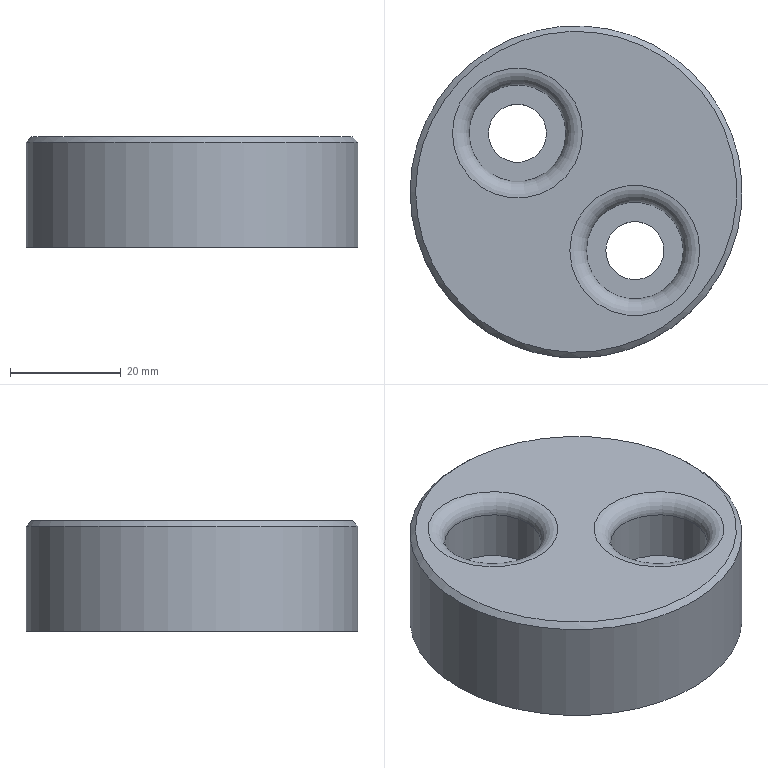Part | NX | features XD1540-60-20 2 | 1 solid | 12 faces | box 60 x 60 x 20 mm | volume 49069 mm3 | cylinder 5 | plane 4 | torus 2 | cone 1 | commonest cylinder face diameters 10.5 x2 17.5 x2 60 x1
STEP:
#1=CARTESIAN_POINT('',(271.,445.,-360.));
#2=VERTEX_POINT('',#1);
#3=CARTESIAN_POINT('',(300.,445.,-360.));
#4=DIRECTION('',(0.,0.,-1.));
#5=DIRECTION('',(-1.,0.,0.));
#6=AXIS2_PLACEMENT_3D('',#3,#4,#5);
#7=CIRCLE('',#6,29.);
#8=EDGE_CURVE('',#2,#2,#7,.T.);
#9=ORIENTED_EDGE('',*,*,#8,.F.);
#10=EDGE_LOOP('',(#9));
#11=FACE_BOUND('',#10,.T.);
#12=CARTESIAN_POINT('',(298.857,434.393,-360.));
#13=VERTEX_POINT('',#12);
#14=CARTESIAN_POINT('',(310.607,434.393,-360.));
#15=DIRECTION('',(0.,0.,1.));
#16=DIRECTION('',(-1.,0.,0.));
#17=AXIS2_PLACEMENT_3D('',#14,#15,#16);
#18=CIRCLE('',#17,11.75);
#19=EDGE_CURVE('',#13,#13,#18,.T.);
#20=ORIENTED_EDGE('',*,*,#19,.F.);
#21=EDGE_LOOP('',(#20));
#22=FACE_BOUND('',#21,.T.);
#23=CARTESIAN_POINT('',(277.643,455.607,-360.));
#24=VERTEX_POINT('',#23);
#25=CARTESIAN_POINT('',(289.393,455.607,-360.));
#26=DIRECTION('',(0.,0.,1.));
#27=DIRECTION('',(-1.,0.,0.));
#28=AXIS2_PLACEMENT_3D('',#25,#26,#27);
#29=CIRCLE('',#28,11.75);
#30=EDGE_CURVE('',#24,#24,#29,.T.);
#31=ORIENTED_EDGE('',*,*,#30,.F.);
#32=EDGE_LOOP('',(#31));
#33=FACE_BOUND('',#32,.T.);
#34=CARTESIAN_POINT('',(300.,445.,-360.));
#35=DIRECTION('',(0.,0.,1.));
#36=DIRECTION('',(1.,0.,0.));
#37=AXIS2_PLACEMENT_3D('',#34,#35,#36);
#38=PLANE('',#37);
#39=ADVANCED_FACE('',(#11,#22,#33),#38,.T.);
#40=CARTESIAN_POINT('',(270.,445.,-380.));
#41=VERTEX_POINT('',#40);
#42=CARTESIAN_POINT('',(300.,445.,-380.));
#43=DIRECTION('',(0.,0.,-1.));
#44=DIRECTION('',(-1.,0.,0.));
#45=AXIS2_PLACEMENT_3D('',#42,#43,#44);
#46=CIRCLE('',#45,30.);
#47=EDGE_CURVE('',#41,#41,#46,.T.);
#48=ORIENTED_EDGE('',*,*,#47,.T.);
#49=EDGE_LOOP('',(#48));
#50=FACE_BOUND('',#49,.T.);
#51=CARTESIAN_POINT('',(315.857,434.393,-380.));
#52=VERTEX_POINT('',#51);
#53=CARTESIAN_POINT('',(310.607,434.393,-380.));
#54=DIRECTION('',(0.,0.,1.));
#55=DIRECTION('',(1.,0.,0.));
#56=AXIS2_PLACEMENT_3D('',#53,#54,#55);
#57=CIRCLE('',#56,5.25);
#58=EDGE_CURVE('',#52,#52,#57,.T.);
#59=ORIENTED_EDGE('',*,*,#58,.T.);
#60=EDGE_LOOP('',(#59));
#61=FACE_BOUND('',#60,.T.);
#62=CARTESIAN_POINT('',(294.643,455.607,-380.));
#63=VERTEX_POINT('',#62);
#64=CARTESIAN_POINT('',(289.393,455.607,-380.));
#65=DIRECTION('',(0.,0.,1.));
#66=DIRECTION('',(1.,0.,0.));
#67=AXIS2_PLACEMENT_3D('',#64,#65,#66);
#68=CIRCLE('',#67,5.25);
#69=EDGE_CURVE('',#63,#63,#68,.T.);
#70=ORIENTED_EDGE('',*,*,#69,.T.);
#71=EDGE_LOOP('',(#70));
#72=FACE_BOUND('',#71,.T.);
#73=CARTESIAN_POINT('',(300.,445.,-380.));
#74=DIRECTION('',(0.,0.,-1.));
#75=DIRECTION('',(-1.,0.,0.));
#76=AXIS2_PLACEMENT_3D('',#73,#74,#75);
#77=PLANE('',#76);
#78=ADVANCED_FACE('',(#50,#61,#72),#77,.T.);
#79=CARTESIAN_POINT('',(325.937,429.925,-361.));
#80=VERTEX_POINT('',#79);
#81=CARTESIAN_POINT('',(300.,445.,-361.));
#82=DIRECTION('',(0.,0.,1.));
#83=DIRECTION('',(-1.,0.,0.));
#84=AXIS2_PLACEMENT_3D('',#81,#82,#83);
#85=CIRCLE('',#84,30.);
#86=EDGE_CURVE('',#80,#80,#85,.T.);
#87=ORIENTED_EDGE('',*,*,#86,.F.);
#88=EDGE_LOOP('',(#87));
#89=FACE_BOUND('',#88,.T.);
#90=ORIENTED_EDGE('',*,*,#47,.F.);
#91=EDGE_LOOP('',(#90));
#92=FACE_BOUND('',#91,.T.);
#93=CARTESIAN_POINT('',(300.,445.,-380.));
#94=DIRECTION('',(0.,0.,1.));
#95=DIRECTION('',(1.,0.,0.));
#96=AXIS2_PLACEMENT_3D('',#93,#94,#95);
#97=CYLINDRICAL_SURFACE('',#96,30.);
#98=ADVANCED_FACE('',(#89,#92),#97,.T.);
#99=CARTESIAN_POINT('',(294.643,455.607,-372.));
#100=VERTEX_POINT('',#99);
#101=CARTESIAN_POINT('',(289.393,455.607,-372.));
#102=DIRECTION('',(0.,0.,1.));
#103=DIRECTION('',(1.,0.,0.));
#104=AXIS2_PLACEMENT_3D('',#101,#102,#103);
#105=CIRCLE('',#104,5.25);
#106=EDGE_CURVE('',#100,#100,#105,.T.);
#107=ORIENTED_EDGE('',*,*,#106,.F.);
#108=EDGE_LOOP('',(#107));
#109=FACE_BOUND('',#108,.T.);
#110=CARTESIAN_POINT('',(280.643,455.607,-372.));
#111=VERTEX_POINT('',#110);
#112=CARTESIAN_POINT('',(289.393,455.607,-372.));
#113=DIRECTION('',(0.,0.,-1.));
#114=DIRECTION('',(-1.,0.,0.));
#115=AXIS2_PLACEMENT_3D('',#112,#113,#114);
#116=CIRCLE('',#115,8.75);
#117=EDGE_CURVE('',#111,#111,#116,.T.);
#118=ORIENTED_EDGE('',*,*,#117,.F.);
#119=EDGE_LOOP('',(#118));
#120=FACE_BOUND('',#119,.T.);
#121=CARTESIAN_POINT('',(289.393,455.607,-372.));
#122=DIRECTION('',(0.,0.,-1.));
#123=DIRECTION('',(-1.,0.,0.));
#124=AXIS2_PLACEMENT_3D('',#121,#122,#123);
#125=PLANE('',#124);
#126=ADVANCED_FACE('',(#109,#120),#125,.F.);
#127=CARTESIAN_POINT('',(280.643,455.607,-363.));
#128=VERTEX_POINT('',#127);
#129=CARTESIAN_POINT('',(289.393,455.607,-363.));
#130=DIRECTION('',(0.,0.,-1.));
#131=DIRECTION('',(-1.,0.,0.));
#132=AXIS2_PLACEMENT_3D('',#129,#130,#131);
#133=CIRCLE('',#132,8.75);
#134=EDGE_CURVE('',#128,#128,#133,.T.);
#135=ORIENTED_EDGE('',*,*,#134,.F.);
#136=EDGE_LOOP('',(#135));
#137=FACE_BOUND('',#136,.T.);
#138=ORIENTED_EDGE('',*,*,#117,.T.);
#139=EDGE_LOOP('',(#138));
#140=FACE_BOUND('',#139,.T.);
#141=CARTESIAN_POINT('',(289.393,455.607,-372.));
#142=DIRECTION('',(0.,0.,1.));
#143=DIRECTION('',(1.,0.,0.));
#144=AXIS2_PLACEMENT_3D('',#141,#142,#143);
#145=CYLINDRICAL_SURFACE('',#144,8.75);
#146=ADVANCED_FACE('',(#137,#140),#145,.F.);
#147=CARTESIAN_POINT('',(315.857,434.393,-372.));
#148=VERTEX_POINT('',#147);
#149=CARTESIAN_POINT('',(310.607,434.393,-372.));
#150=DIRECTION('',(0.,0.,1.));
#151=DIRECTION('',(1.,0.,0.));
#152=AXIS2_PLACEMENT_3D('',#149,#150,#151);
#153=CIRCLE('',#152,5.25);
#154=EDGE_CURVE('',#148,#148,#153,.T.);
#155=ORIENTED_EDGE('',*,*,#154,.F.);
#156=EDGE_LOOP('',(#155));
#157=FACE_BOUND('',#156,.T.);
#158=CARTESIAN_POINT('',(301.857,434.393,-372.));
#159=VERTEX_POINT('',#158);
#160=CARTESIAN_POINT('',(310.607,434.393,-372.));
#161=DIRECTION('',(0.,0.,-1.));
#162=DIRECTION('',(-1.,0.,0.));
#163=AXIS2_PLACEMENT_3D('',#160,#161,#162);
#164=CIRCLE('',#163,8.75);
#165=EDGE_CURVE('',#159,#159,#164,.T.);
#166=ORIENTED_EDGE('',*,*,#165,.F.);
#167=EDGE_LOOP('',(#166));
#168=FACE_BOUND('',#167,.T.);
#169=CARTESIAN_POINT('',(310.607,434.393,-372.));
#170=DIRECTION('',(0.,0.,-1.));
#171=DIRECTION('',(-1.,0.,0.));
#172=AXIS2_PLACEMENT_3D('',#169,#170,#171);
#173=PLANE('',#172);
#174=ADVANCED_FACE('',(#157,#168),#173,.F.);
#175=CARTESIAN_POINT('',(301.857,434.393,-363.));
#176=VERTEX_POINT('',#175);
#177=CARTESIAN_POINT('',(310.607,434.393,-363.));
#178=DIRECTION('',(0.,0.,-1.));
#179=DIRECTION('',(-1.,0.,0.));
#180=AXIS2_PLACEMENT_3D('',#177,#178,#179);
#181=CIRCLE('',#180,8.75);
#182=EDGE_CURVE('',#176,#176,#181,.T.);
#183=ORIENTED_EDGE('',*,*,#182,.F.);
#184=EDGE_LOOP('',(#183));
#185=FACE_BOUND('',#184,.T.);
#186=ORIENTED_EDGE('',*,*,#165,.T.);
#187=EDGE_LOOP('',(#186));
#188=FACE_BOUND('',#187,.T.);
#189=CARTESIAN_POINT('',(310.607,434.393,-372.));
#190=DIRECTION('',(0.,0.,1.));
#191=DIRECTION('',(1.,0.,0.));
#192=AXIS2_PLACEMENT_3D('',#189,#190,#191);
#193=CYLINDRICAL_SURFACE('',#192,8.75);
#194=ADVANCED_FACE('',(#185,#188),#193,.F.);
#195=ORIENTED_EDGE('',*,*,#69,.F.);
#196=EDGE_LOOP('',(#195));
#197=FACE_BOUND('',#196,.T.);
#198=ORIENTED_EDGE('',*,*,#106,.T.);
#199=EDGE_LOOP('',(#198));
#200=FACE_BOUND('',#199,.T.);
#201=CARTESIAN_POINT('',(289.393,455.607,-381.));
#202=DIRECTION('',(0.,0.,1.));
#203=DIRECTION('',(1.,0.,0.));
#204=AXIS2_PLACEMENT_3D('',#201,#202,#203);
#205=CYLINDRICAL_SURFACE('',#204,5.25);
#206=ADVANCED_FACE('',(#197,#200),#205,.F.);
#207=ORIENTED_EDGE('',*,*,#58,.F.);
#208=EDGE_LOOP('',(#207));
#209=FACE_BOUND('',#208,.T.);
#210=ORIENTED_EDGE('',*,*,#154,.T.);
#211=EDGE_LOOP('',(#210));
#212=FACE_BOUND('',#211,.T.);
#213=CARTESIAN_POINT('',(310.607,434.393,-381.));
#214=DIRECTION('',(0.,0.,1.));
#215=DIRECTION('',(1.,0.,0.));
#216=AXIS2_PLACEMENT_3D('',#213,#214,#215);
#217=CYLINDRICAL_SURFACE('',#216,5.25);
#218=ADVANCED_FACE('',(#209,#212),#217,.F.);
#219=ORIENTED_EDGE('',*,*,#30,.T.);
#220=EDGE_LOOP('',(#219));
#221=FACE_BOUND('',#220,.T.);
#222=ORIENTED_EDGE('',*,*,#134,.T.);
#223=EDGE_LOOP('',(#222));
#224=FACE_BOUND('',#223,.T.);
#225=CARTESIAN_POINT('',(289.393,455.607,-363.));
#226=DIRECTION('',(0.,0.,1.));
#227=DIRECTION('',(1.,0.,0.));
#228=AXIS2_PLACEMENT_3D('',#225,#226,#227);
#229=TOROIDAL_SURFACE('',#228,11.75,3.);
#230=ADVANCED_FACE('',(#221,#224),#229,.T.);
#231=ORIENTED_EDGE('',*,*,#19,.T.);
#232=EDGE_LOOP('',(#231));
#233=FACE_BOUND('',#232,.T.);
#234=ORIENTED_EDGE('',*,*,#182,.T.);
#235=EDGE_LOOP('',(#234));
#236=FACE_BOUND('',#235,.T.);
#237=CARTESIAN_POINT('',(310.607,434.393,-363.));
#238=DIRECTION('',(0.,0.,1.));
#239=DIRECTION('',(1.,0.,0.));
#240=AXIS2_PLACEMENT_3D('',#237,#238,#239);
#241=TOROIDAL_SURFACE('',#240,11.75,3.);
#242=ADVANCED_FACE('',(#233,#236),#241,.T.);
#243=ORIENTED_EDGE('',*,*,#86,.T.);
#244=EDGE_LOOP('',(#243));
#245=FACE_BOUND('',#244,.T.);
#246=ORIENTED_EDGE('',*,*,#8,.T.);
#247=EDGE_LOOP('',(#246));
#248=FACE_BOUND('',#247,.T.);
#249=CARTESIAN_POINT('',(300.,445.,-361.));
#250=DIRECTION('',(0.,0.,-1.));
#251=DIRECTION('',(-1.,0.,0.));
#252=AXIS2_PLACEMENT_3D('',#249,#250,#251);
#253=CONICAL_SURFACE('',#252,30.,0.7854);
#254=ADVANCED_FACE('',(#245,#248),#253,.T.);
#255=CLOSED_SHELL('',(#39,#78,#98,#126,#146,#174,#194,#206,#218,#230,#242,#254));
#256=MANIFOLD_SOLID_BREP('',#255);
#257=(LENGTH_UNIT()NAMED_UNIT(*)SI_UNIT(.MILLI.,.METRE.));
#258=UNCERTAINTY_MEASURE_WITH_UNIT(LENGTH_MEASURE(0.00001),#257,'','');
#259=(NAMED_UNIT(*)PLANE_ANGLE_UNIT()SI_UNIT($,.RADIAN.));
#260=(NAMED_UNIT(*)SI_UNIT($,.STERADIAN.)SOLID_ANGLE_UNIT());
#261=(GEOMETRIC_REPRESENTATION_CONTEXT(3)GLOBAL_UNCERTAINTY_ASSIGNED_CONTEXT((#258))GLOBAL_UNIT_ASSIGNED_CONTEXT((#257,#259,#260))REPRESENTATION_CONTEXT('',''));
#262=ADVANCED_BREP_SHAPE_REPRESENTATION('',(#256),#261);